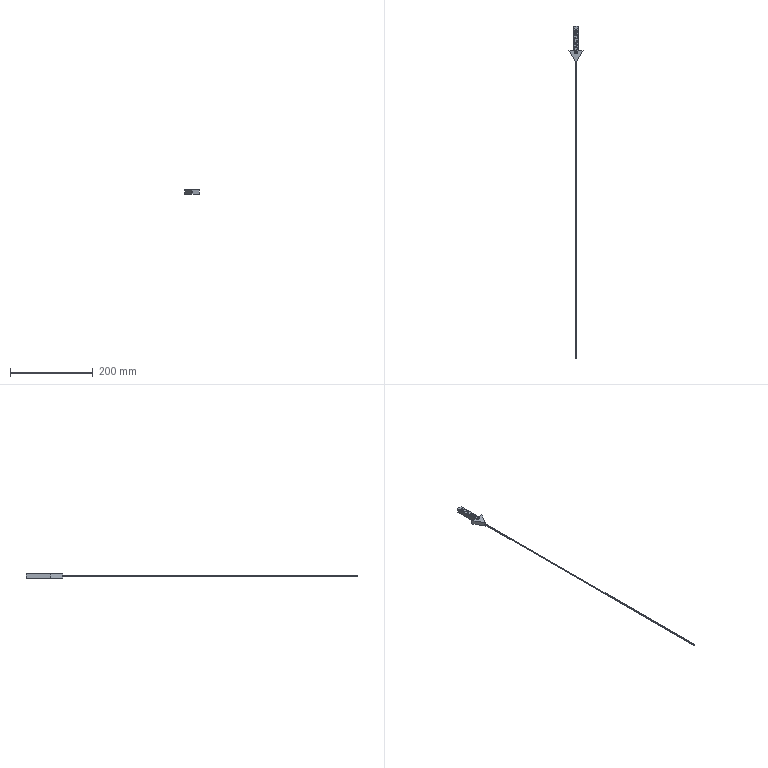Part | STEP file | lll_id1602_x_t | 1 solid | 126 faces | box 34.103 x 804.766 x 10 mm | volume 15071 mm3 | plane 94 | other 32